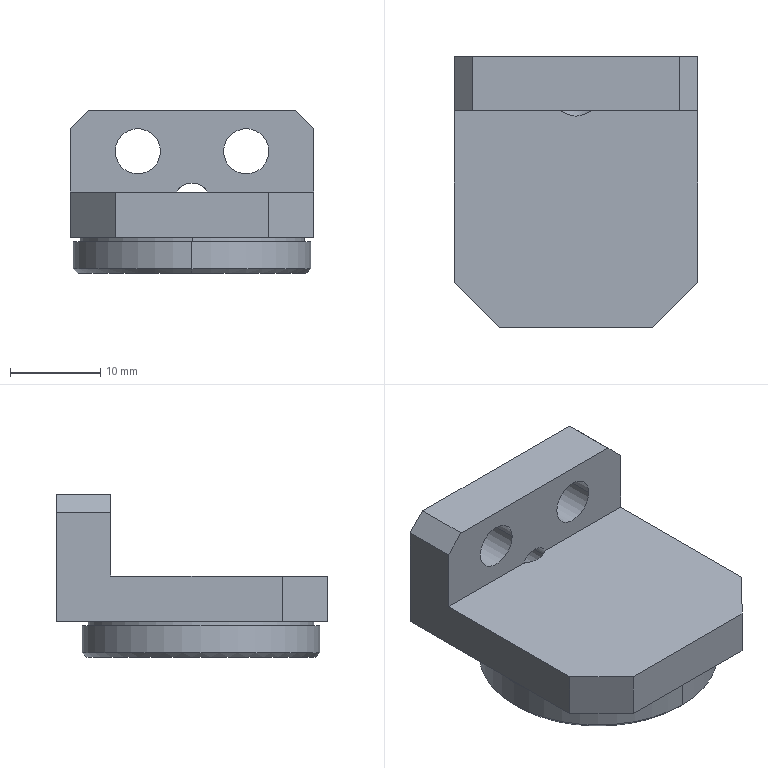Part | NX | 1 solid | 28 faces | box 27 x 30 x 18 mm | volume 7179 mm3 | plane 14 | cylinder 10 | cone 4 | commonest cylinder face diameters 5 x4 4 x2 25 x2 26.29 x2
STEP:
#1=CARTESIAN_POINT('',(0.,0.145,-17.5));
#2=VERTEX_POINT('',#1);
#3=CARTESIAN_POINT('',(0.,-26.145,-17.5));
#4=VERTEX_POINT('',#3);
#5=CARTESIAN_POINT('',(0.,-13.,-17.5));
#6=DIRECTION('',(0.,0.,1.));
#7=DIRECTION('',(0.,-1.,0.));
#8=AXIS2_PLACEMENT_3D('',#5,#6,#7);
#9=CIRCLE('',#8,13.145);
#10=EDGE_CURVE('',#2,#4,#9,.T.);
#11=ORIENTED_EDGE('',*,*,#10,.T.);
#12=CARTESIAN_POINT('',(0.,-26.145,-14.5));
#13=VERTEX_POINT('',#12);
#14=CARTESIAN_POINT('',(0.,-26.145,-18.));
#15=DIRECTION('',(0.,0.,1.));
#16=VECTOR('',#15,1000.);
#17=LINE('',#14,#16);
#18=EDGE_CURVE('',#13,#4,#17,.F.);
#19=ORIENTED_EDGE('',*,*,#18,.F.);
#20=CARTESIAN_POINT('',(0.,0.145,-14.5));
#21=VERTEX_POINT('',#20);
#22=CARTESIAN_POINT('',(0.,-13.,-14.5));
#23=DIRECTION('',(0.,0.,-1.));
#24=DIRECTION('',(0.,-1.,0.));
#25=AXIS2_PLACEMENT_3D('',#22,#23,#24);
#26=CIRCLE('',#25,13.145);
#27=EDGE_CURVE('',#13,#21,#26,.T.);
#28=ORIENTED_EDGE('',*,*,#27,.T.);
#29=CARTESIAN_POINT('',(0.,0.145,-18.));
#30=DIRECTION('',(0.,0.,1.));
#31=VECTOR('',#30,1000.);
#32=LINE('',#29,#31);
#33=EDGE_CURVE('',#21,#2,#32,.F.);
#34=ORIENTED_EDGE('',*,*,#33,.T.);
#35=EDGE_LOOP('',(#11,#19,#28,#34));
#36=FACE_BOUND('',#35,.T.);
#37=CARTESIAN_POINT('',(0.,-13.,-18.));
#38=DIRECTION('',(0.,0.,1.));
#39=DIRECTION('',(0.,-1.,0.));
#40=AXIS2_PLACEMENT_3D('',#37,#38,#39);
#41=CYLINDRICAL_SURFACE('',#40,13.145);
#42=ADVANCED_FACE('',(#36),#41,.T.);
#43=CARTESIAN_POINT('',(0.,-25.645,-18.));
#44=VERTEX_POINT('',#43);
#45=CARTESIAN_POINT('',(0.,-0.355,-18.));
#46=VERTEX_POINT('',#45);
#47=CARTESIAN_POINT('',(0.,-13.,-18.));
#48=DIRECTION('',(0.,0.,-1.));
#49=DIRECTION('',(0.,-1.,0.));
#50=AXIS2_PLACEMENT_3D('',#47,#48,#49);
#51=CIRCLE('',#50,12.645);
#52=EDGE_CURVE('',#44,#46,#51,.T.);
#53=ORIENTED_EDGE('',*,*,#52,.F.);
#54=CARTESIAN_POINT('',(0.,-25.645,-18.));
#55=DIRECTION('',(0.,-0.7071,0.7071));
#56=VECTOR('',#55,1000.);
#57=LINE('',#54,#56);
#58=EDGE_CURVE('',#4,#44,#57,.F.);
#59=ORIENTED_EDGE('',*,*,#58,.F.);
#60=ORIENTED_EDGE('',*,*,#10,.F.);
#61=CARTESIAN_POINT('',(0.,-0.355,-18.));
#62=DIRECTION('',(0.,0.7071,0.7071));
#63=VECTOR('',#62,1000.);
#64=LINE('',#61,#63);
#65=EDGE_CURVE('',#2,#46,#64,.F.);
#66=ORIENTED_EDGE('',*,*,#65,.T.);
#67=EDGE_LOOP('',(#53,#59,#60,#66));
#68=FACE_BOUND('',#67,.T.);
#69=CARTESIAN_POINT('',(0.,-13.,-18.));
#70=DIRECTION('',(0.,0.,1.));
#71=DIRECTION('',(0.,-1.,0.));
#72=AXIS2_PLACEMENT_3D('',#69,#70,#71);
#73=CONICAL_SURFACE('',#72,12.645,0.7854);
#74=ADVANCED_FACE('',(#68),#73,.T.);
#75=CARTESIAN_POINT('',(0.,-25.5,-14.5));
#76=VERTEX_POINT('',#75);
#77=CARTESIAN_POINT('',(0.,-0.5,-14.5));
#78=VERTEX_POINT('',#77);
#79=CARTESIAN_POINT('',(0.,-13.,-14.5));
#80=DIRECTION('',(0.,0.,-1.));
#81=DIRECTION('',(0.,-1.,0.));
#82=AXIS2_PLACEMENT_3D('',#79,#80,#81);
#83=CIRCLE('',#82,12.5);
#84=EDGE_CURVE('',#76,#78,#83,.T.);
#85=ORIENTED_EDGE('',*,*,#84,.F.);
#86=CARTESIAN_POINT('',(0.,-25.5,-14.));
#87=VERTEX_POINT('',#86);
#88=CARTESIAN_POINT('',(0.,-25.5,-14.5));
#89=DIRECTION('',(0.,0.,1.));
#90=VECTOR('',#89,1000.);
#91=LINE('',#88,#90);
#92=EDGE_CURVE('',#87,#76,#91,.F.);
#93=ORIENTED_EDGE('',*,*,#92,.F.);
#94=CARTESIAN_POINT('',(0.,-0.5,-14.));
#95=VERTEX_POINT('',#94);
#96=CARTESIAN_POINT('',(0.,-13.,-14.));
#97=DIRECTION('',(0.,0.,-1.));
#98=DIRECTION('',(0.,-1.,0.));
#99=AXIS2_PLACEMENT_3D('',#96,#97,#98);
#100=CIRCLE('',#99,12.5);
#101=EDGE_CURVE('',#87,#95,#100,.T.);
#102=ORIENTED_EDGE('',*,*,#101,.T.);
#103=CARTESIAN_POINT('',(0.,-0.5,-14.5));
#104=DIRECTION('',(0.,0.,1.));
#105=VECTOR('',#104,1000.);
#106=LINE('',#103,#105);
#107=EDGE_CURVE('',#95,#78,#106,.F.);
#108=ORIENTED_EDGE('',*,*,#107,.T.);
#109=EDGE_LOOP('',(#85,#93,#102,#108));
#110=FACE_BOUND('',#109,.T.);
#111=CARTESIAN_POINT('',(0.,-13.,-14.5));
#112=DIRECTION('',(0.,0.,1.));
#113=DIRECTION('',(0.,-1.,0.));
#114=AXIS2_PLACEMENT_3D('',#111,#112,#113);
#115=CYLINDRICAL_SURFACE('',#114,12.5);
#116=ADVANCED_FACE('',(#110),#115,.T.);
#117=CARTESIAN_POINT('',(-2.,-3.,-10.));
#118=VERTEX_POINT('',#117);
#119=CARTESIAN_POINT('',(-1.732,-3.,-9.));
#120=VERTEX_POINT('',#119);
#121=CARTESIAN_POINT('',(0.,-3.,-10.));
#122=DIRECTION('',(0.,1.,0.));
#123=DIRECTION('',(1.,0.,0.));
#124=AXIS2_PLACEMENT_3D('',#121,#122,#123);
#125=CIRCLE('',#124,2.);
#126=EDGE_CURVE('',#118,#120,#125,.T.);
#127=ORIENTED_EDGE('',*,*,#126,.F.);
#128=CARTESIAN_POINT('',(-2.,3.,-10.));
#129=VERTEX_POINT('',#128);
#130=CARTESIAN_POINT('',(-2.,3.,-10.));
#131=DIRECTION('',(0.,1.,0.));
#132=VECTOR('',#131,1000.);
#133=LINE('',#130,#132);
#134=EDGE_CURVE('',#129,#118,#133,.F.);
#135=ORIENTED_EDGE('',*,*,#134,.F.);
#136=CARTESIAN_POINT('',(2.,3.,-10.));
#137=VERTEX_POINT('',#136);
#138=CARTESIAN_POINT('',(0.,3.,-10.));
#139=DIRECTION('',(0.,1.,0.));
#140=DIRECTION('',(1.,0.,0.));
#141=AXIS2_PLACEMENT_3D('',#138,#139,#140);
#142=CIRCLE('',#141,2.);
#143=EDGE_CURVE('',#129,#137,#142,.T.);
#144=ORIENTED_EDGE('',*,*,#143,.T.);
#145=CARTESIAN_POINT('',(2.,-3.,-10.));
#146=VERTEX_POINT('',#145);
#147=CARTESIAN_POINT('',(2.,3.,-10.));
#148=DIRECTION('',(0.,1.,0.));
#149=VECTOR('',#148,1000.);
#150=LINE('',#147,#149);
#151=EDGE_CURVE('',#137,#146,#150,.F.);
#152=ORIENTED_EDGE('',*,*,#151,.T.);
#153=CARTESIAN_POINT('',(1.732,-3.,-9.));
#154=VERTEX_POINT('',#153);
#155=CARTESIAN_POINT('',(0.,-3.,-10.));
#156=DIRECTION('',(0.,1.,0.));
#157=DIRECTION('',(1.,0.,0.));
#158=AXIS2_PLACEMENT_3D('',#155,#156,#157);
#159=CIRCLE('',#158,2.);
#160=EDGE_CURVE('',#154,#146,#159,.T.);
#161=ORIENTED_EDGE('',*,*,#160,.F.);
#162=CARTESIAN_POINT('',(0.,-3.,-10.));
#163=DIRECTION('',(0.,1.,0.));
#164=DIRECTION('',(1.,0.,0.));
#165=AXIS2_PLACEMENT_3D('',#162,#163,#164);
#166=CIRCLE('',#165,2.);
#167=EDGE_CURVE('',#120,#154,#166,.T.);
#168=ORIENTED_EDGE('',*,*,#167,.F.);
#169=EDGE_LOOP('',(#127,#135,#144,#152,#161,#168));
#170=FACE_BOUND('',#169,.T.);
#171=CARTESIAN_POINT('',(0.,3.,-10.));
#172=DIRECTION('',(0.,1.,0.));
#173=DIRECTION('',(-1.,0.,0.));
#174=AXIS2_PLACEMENT_3D('',#171,#172,#173);
#175=CYLINDRICAL_SURFACE('',#174,2.);
#176=ADVANCED_FACE('',(#170),#175,.F.);
#177=CARTESIAN_POINT('',(0.,-4.202,-10.));
#178=VERTEX_POINT('',#177);
#179=CARTESIAN_POINT('',(2.,-3.,-10.));
#180=DIRECTION('',(0.8572,0.515,0.));
#181=VECTOR('',#180,1000.);
#182=LINE('',#179,#181);
#183=EDGE_CURVE('',#146,#178,#182,.F.);
#184=ORIENTED_EDGE('',*,*,#183,.T.);
#185=CARTESIAN_POINT('',(-2.,-3.,-10.));
#186=DIRECTION('',(-0.8572,0.515,0.));
#187=VECTOR('',#186,1000.);
#188=LINE('',#185,#187);
#189=EDGE_CURVE('',#118,#178,#188,.F.);
#190=ORIENTED_EDGE('',*,*,#189,.F.);
#191=ORIENTED_EDGE('',*,*,#126,.T.);
#192=CARTESIAN_POINT('',(1.732,-3.,-9.));
#193=CARTESIAN_POINT('',(1.184,-3.285,-9.));
#194=CARTESIAN_POINT('',(-0.003576,-3.917,-9.));
#195=CARTESIAN_POINT('',(-1.185,-3.285,-9.));
#196=CARTESIAN_POINT('',(-1.732,-3.,-9.));
#197=B_SPLINE_CURVE_WITH_KNOTS('',3,(#192,#193,#194,#195,#196),.UNSPECIFIED.,.F.,.F.,(4,1,4),(0.,0.001852,0.003703),.UNSPECIFIED.);
#198=EDGE_CURVE('',#154,#120,#197,.T.);
#199=ORIENTED_EDGE('',*,*,#198,.F.);
#200=ORIENTED_EDGE('',*,*,#160,.T.);
#201=EDGE_LOOP('',(#184,#190,#191,#199,#200));
#202=FACE_BOUND('',#201,.T.);
#203=CARTESIAN_POINT('',(0.,-3.,-10.));
#204=DIRECTION('',(0.,1.,0.));
#205=DIRECTION('',(-1.,0.,0.));
#206=AXIS2_PLACEMENT_3D('',#203,#204,#205);
#207=CONICAL_SURFACE('',#206,2.,1.03);
#208=ADVANCED_FACE('',(#202),#207,.F.);
#209=CARTESIAN_POINT('',(-8.5,-3.,-4.5));
#210=VERTEX_POINT('',#209);
#211=CARTESIAN_POINT('',(-3.5,-3.,-4.5));
#212=VERTEX_POINT('',#211);
#213=CARTESIAN_POINT('',(-6.,-3.,-4.5));
#214=DIRECTION('',(0.,1.,0.));
#215=DIRECTION('',(1.,0.,0.));
#216=AXIS2_PLACEMENT_3D('',#213,#214,#215);
#217=CIRCLE('',#216,2.5);
#218=EDGE_CURVE('',#210,#212,#217,.T.);
#219=ORIENTED_EDGE('',*,*,#218,.F.);
#220=CARTESIAN_POINT('',(-8.5,3.,-4.5));
#221=VERTEX_POINT('',#220);
#222=CARTESIAN_POINT('',(-8.5,-6.,-4.5));
#223=DIRECTION('',(0.,1.,0.));
#224=VECTOR('',#223,1000.);
#225=LINE('',#222,#224);
#226=EDGE_CURVE('',#221,#210,#225,.F.);
#227=ORIENTED_EDGE('',*,*,#226,.F.);
#228=CARTESIAN_POINT('',(-3.5,3.,-4.5));
#229=VERTEX_POINT('',#228);
#230=CARTESIAN_POINT('',(-6.,3.,-4.5));
#231=DIRECTION('',(0.,1.,0.));
#232=DIRECTION('',(1.,0.,0.));
#233=AXIS2_PLACEMENT_3D('',#230,#231,#232);
#234=CIRCLE('',#233,2.5);
#235=EDGE_CURVE('',#221,#229,#234,.T.);
#236=ORIENTED_EDGE('',*,*,#235,.T.);
#237=CARTESIAN_POINT('',(-3.5,-6.,-4.5));
#238=DIRECTION('',(0.,1.,0.));
#239=VECTOR('',#238,1000.);
#240=LINE('',#237,#239);
#241=EDGE_CURVE('',#229,#212,#240,.F.);
#242=ORIENTED_EDGE('',*,*,#241,.T.);
#243=EDGE_LOOP('',(#219,#227,#236,#242));
#244=FACE_BOUND('',#243,.T.);
#245=CARTESIAN_POINT('',(-6.,-6.,-4.5));
#246=DIRECTION('',(0.,1.,0.));
#247=DIRECTION('',(-1.,0.,0.));
#248=AXIS2_PLACEMENT_3D('',#245,#246,#247);
#249=CYLINDRICAL_SURFACE('',#248,2.5);
#250=ADVANCED_FACE('',(#244),#249,.F.);
#251=CARTESIAN_POINT('',(3.5,-3.,-4.5));
#252=VERTEX_POINT('',#251);
#253=CARTESIAN_POINT('',(8.5,-3.,-4.5));
#254=VERTEX_POINT('',#253);
#255=CARTESIAN_POINT('',(6.,-3.,-4.5));
#256=DIRECTION('',(0.,1.,0.));
#257=DIRECTION('',(1.,0.,0.));
#258=AXIS2_PLACEMENT_3D('',#255,#256,#257);
#259=CIRCLE('',#258,2.5);
#260=EDGE_CURVE('',#252,#254,#259,.T.);
#261=ORIENTED_EDGE('',*,*,#260,.F.);
#262=CARTESIAN_POINT('',(3.5,3.,-4.5));
#263=VERTEX_POINT('',#262);
#264=CARTESIAN_POINT('',(3.5,-6.,-4.5));
#265=DIRECTION('',(0.,1.,0.));
#266=VECTOR('',#265,1000.);
#267=LINE('',#264,#266);
#268=EDGE_CURVE('',#263,#252,#267,.F.);
#269=ORIENTED_EDGE('',*,*,#268,.F.);
#270=CARTESIAN_POINT('',(8.5,3.,-4.5));
#271=VERTEX_POINT('',#270);
#272=CARTESIAN_POINT('',(6.,3.,-4.5));
#273=DIRECTION('',(0.,1.,0.));
#274=DIRECTION('',(1.,0.,0.));
#275=AXIS2_PLACEMENT_3D('',#272,#273,#274);
#276=CIRCLE('',#275,2.5);
#277=EDGE_CURVE('',#263,#271,#276,.T.);
#278=ORIENTED_EDGE('',*,*,#277,.T.);
#279=CARTESIAN_POINT('',(8.5,-6.,-4.5));
#280=DIRECTION('',(0.,1.,0.));
#281=VECTOR('',#280,1000.);
#282=LINE('',#279,#281);
#283=EDGE_CURVE('',#271,#254,#282,.F.);
#284=ORIENTED_EDGE('',*,*,#283,.T.);
#285=EDGE_LOOP('',(#261,#269,#278,#284));
#286=FACE_BOUND('',#285,.T.);
#287=CARTESIAN_POINT('',(6.,-6.,-4.5));
#288=DIRECTION('',(0.,1.,0.));
#289=DIRECTION('',(-1.,0.,0.));
#290=AXIS2_PLACEMENT_3D('',#287,#288,#289);
#291=CYLINDRICAL_SURFACE('',#290,2.5);
#292=ADVANCED_FACE('',(#286),#291,.F.);
#293=CARTESIAN_POINT('',(-13.5,-22.,-9.));
#294=VERTEX_POINT('',#293);
#295=CARTESIAN_POINT('',(-13.5,-3.,-9.));
#296=VERTEX_POINT('',#295);
#297=CARTESIAN_POINT('',(-13.5,-27.,-9.));
#298=DIRECTION('',(0.,1.,0.));
#299=VECTOR('',#298,1000.);
#300=LINE('',#297,#299);
#301=EDGE_CURVE('',#294,#296,#300,.T.);
#302=ORIENTED_EDGE('',*,*,#301,.F.);
#303=CARTESIAN_POINT('',(-8.5,-27.,-9.));
#304=VERTEX_POINT('',#303);
#305=CARTESIAN_POINT('',(-13.5,-22.,-9.));
#306=DIRECTION('',(0.7071,-0.7071,0.));
#307=VECTOR('',#306,1000.);
#308=LINE('',#305,#307);
#309=EDGE_CURVE('',#294,#304,#308,.T.);
#310=ORIENTED_EDGE('',*,*,#309,.T.);
#311=CARTESIAN_POINT('',(8.5,-27.,-9.));
#312=VERTEX_POINT('',#311);
#313=CARTESIAN_POINT('',(-13.5,-27.,-9.));
#314=DIRECTION('',(-1.,0.,0.));
#315=VECTOR('',#314,1000.);
#316=LINE('',#313,#315);
#317=EDGE_CURVE('',#312,#304,#316,.T.);
#318=ORIENTED_EDGE('',*,*,#317,.F.);
#319=CARTESIAN_POINT('',(13.5,-22.,-9.));
#320=VERTEX_POINT('',#319);
#321=CARTESIAN_POINT('',(8.5,-27.,-9.));
#322=DIRECTION('',(0.7071,0.7071,0.));
#323=VECTOR('',#322,1000.);
#324=LINE('',#321,#323);
#325=EDGE_CURVE('',#312,#320,#324,.T.);
#326=ORIENTED_EDGE('',*,*,#325,.T.);
#327=CARTESIAN_POINT('',(13.5,-3.,-9.));
#328=VERTEX_POINT('',#327);
#329=CARTESIAN_POINT('',(13.5,-27.,-9.));
#330=DIRECTION('',(0.,-1.,0.));
#331=VECTOR('',#330,1000.);
#332=LINE('',#329,#331);
#333=EDGE_CURVE('',#328,#320,#332,.T.);
#334=ORIENTED_EDGE('',*,*,#333,.F.);
#335=CARTESIAN_POINT('',(13.5,-3.,-9.));
#336=DIRECTION('',(1.,0.,0.));
#337=VECTOR('',#336,1000.);
#338=LINE('',#335,#337);
#339=EDGE_CURVE('',#154,#328,#338,.T.);
#340=ORIENTED_EDGE('',*,*,#339,.F.);
#341=ORIENTED_EDGE('',*,*,#198,.T.);
#342=CARTESIAN_POINT('',(13.5,-3.,-9.));
#343=DIRECTION('',(1.,0.,0.));
#344=VECTOR('',#343,1000.);
#345=LINE('',#342,#344);
#346=EDGE_CURVE('',#296,#120,#345,.T.);
#347=ORIENTED_EDGE('',*,*,#346,.F.);
#348=EDGE_LOOP('',(#302,#310,#318,#326,#334,#340,#341,#347));
#349=FACE_BOUND('',#348,.T.);
#350=CARTESIAN_POINT('',(0.,-13.,-9.));
#351=DIRECTION('',(0.,0.,-1.));
#352=DIRECTION('',(0.,1.,0.));
#353=AXIS2_PLACEMENT_3D('',#350,#351,#352);
#354=PLANE('',#353);
#355=ADVANCED_FACE('',(#349),#354,.F.);
#356=ORIENTED_EDGE('',*,*,#333,.T.);
#357=CARTESIAN_POINT('',(13.5,-22.,-14.));
#358=VERTEX_POINT('',#357);
#359=CARTESIAN_POINT('',(13.5,-22.,-14.));
#360=DIRECTION('',(0.,0.,-1.));
#361=VECTOR('',#360,1000.);
#362=LINE('',#359,#361);
#363=EDGE_CURVE('',#320,#358,#362,.T.);
#364=ORIENTED_EDGE('',*,*,#363,.T.);
#365=CARTESIAN_POINT('',(13.5,3.,-14.));
#366=VERTEX_POINT('',#365);
#367=CARTESIAN_POINT('',(13.5,-27.,-14.));
#368=DIRECTION('',(0.,-1.,0.));
#369=VECTOR('',#368,1000.);
#370=LINE('',#367,#369);
#371=EDGE_CURVE('',#366,#358,#370,.T.);
#372=ORIENTED_EDGE('',*,*,#371,.F.);
#373=CARTESIAN_POINT('',(13.5,3.,-2.));
#374=VERTEX_POINT('',#373);
#375=CARTESIAN_POINT('',(13.5,3.,-14.));
#376=DIRECTION('',(0.,0.,1.));
#377=VECTOR('',#376,1000.);
#378=LINE('',#375,#377);
#379=EDGE_CURVE('',#366,#374,#378,.T.);
#380=ORIENTED_EDGE('',*,*,#379,.T.);
#381=CARTESIAN_POINT('',(13.5,-3.,-2.));
#382=VERTEX_POINT('',#381);
#383=CARTESIAN_POINT('',(13.5,-27.,-2.));
#384=DIRECTION('',(0.,-1.,0.));
#385=VECTOR('',#384,1000.);
#386=LINE('',#383,#385);
#387=EDGE_CURVE('',#374,#382,#386,.T.);
#388=ORIENTED_EDGE('',*,*,#387,.T.);
#389=CARTESIAN_POINT('',(13.5,-3.,0.));
#390=DIRECTION('',(0.,0.,-1.));
#391=VECTOR('',#390,1000.);
#392=LINE('',#389,#391);
#393=EDGE_CURVE('',#382,#328,#392,.T.);
#394=ORIENTED_EDGE('',*,*,#393,.T.);
#395=EDGE_LOOP('',(#356,#364,#372,#380,#388,#394));
#396=FACE_BOUND('',#395,.T.);
#397=CARTESIAN_POINT('',(13.5,-27.,-14.));
#398=DIRECTION('',(-1.,0.,0.));
#399=DIRECTION('',(0.,-1.,0.));
#400=AXIS2_PLACEMENT_3D('',#397,#398,#399);
#401=PLANE('',#400);
#402=ADVANCED_FACE('',(#396),#401,.F.);
#403=ORIENTED_EDGE('',*,*,#317,.T.);
#404=CARTESIAN_POINT('',(-8.5,-27.,-14.));
#405=VERTEX_POINT('',#404);
#406=CARTESIAN_POINT('',(-8.5,-27.,-14.));
#407=DIRECTION('',(0.,0.,-1.));
#408=VECTOR('',#407,1000.);
#409=LINE('',#406,#408);
#410=EDGE_CURVE('',#304,#405,#409,.T.);
#411=ORIENTED_EDGE('',*,*,#410,.T.);
#412=CARTESIAN_POINT('',(8.5,-27.,-14.));
#413=VERTEX_POINT('',#412);
#414=CARTESIAN_POINT('',(-13.5,-27.,-14.));
#415=DIRECTION('',(-1.,0.,0.));
#416=VECTOR('',#415,1000.);
#417=LINE('',#414,#416);
#418=EDGE_CURVE('',#413,#405,#417,.T.);
#419=ORIENTED_EDGE('',*,*,#418,.F.);
#420=CARTESIAN_POINT('',(8.5,-27.,-14.));
#421=DIRECTION('',(0.,0.,1.));
#422=VECTOR('',#421,1000.);
#423=LINE('',#420,#422);
#424=EDGE_CURVE('',#413,#312,#423,.T.);
#425=ORIENTED_EDGE('',*,*,#424,.T.);
#426=EDGE_LOOP('',(#403,#411,#419,#425));
#427=FACE_BOUND('',#426,.T.);
#428=CARTESIAN_POINT('',(-13.5,-27.,-14.));
#429=DIRECTION('',(0.,1.,0.));
#430=DIRECTION('',(-1.,0.,0.));
#431=AXIS2_PLACEMENT_3D('',#428,#429,#430);
#432=PLANE('',#431);
#433=ADVANCED_FACE('',(#427),#432,.F.);
#434=CARTESIAN_POINT('',(-13.5,-22.,-14.));
#435=VERTEX_POINT('',#434);
#436=CARTESIAN_POINT('',(-13.5,3.,-14.));
#437=VERTEX_POINT('',#436);
#438=CARTESIAN_POINT('',(-13.5,-27.,-14.));
#439=DIRECTION('',(0.,1.,0.));
#440=VECTOR('',#439,1000.);
#441=LINE('',#438,#440);
#442=EDGE_CURVE('',#435,#437,#441,.T.);
#443=ORIENTED_EDGE('',*,*,#442,.F.);
#444=CARTESIAN_POINT('',(-13.5,-22.,-14.));
#445=DIRECTION('',(0.,0.,1.));
#446=VECTOR('',#445,1000.);
#447=LINE('',#444,#446);
#448=EDGE_CURVE('',#435,#294,#447,.T.);
#449=ORIENTED_EDGE('',*,*,#448,.T.);
#450=ORIENTED_EDGE('',*,*,#301,.T.);
#451=CARTESIAN_POINT('',(-13.5,-3.,-2.));
#452=VERTEX_POINT('',#451);
#453=CARTESIAN_POINT('',(-13.5,-3.,0.));
#454=DIRECTION('',(0.,0.,-1.));
#455=VECTOR('',#454,1000.);
#456=LINE('',#453,#455);
#457=EDGE_CURVE('',#452,#296,#456,.T.);
#458=ORIENTED_EDGE('',*,*,#457,.F.);
#459=CARTESIAN_POINT('',(-13.5,3.,-2.));
#460=VERTEX_POINT('',#459);
#461=CARTESIAN_POINT('',(-13.5,-27.,-2.));
#462=DIRECTION('',(0.,1.,0.));
#463=VECTOR('',#462,1000.);
#464=LINE('',#461,#463);
#465=EDGE_CURVE('',#452,#460,#464,.T.);
#466=ORIENTED_EDGE('',*,*,#465,.T.);
#467=CARTESIAN_POINT('',(-13.5,3.,-14.));
#468=DIRECTION('',(0.,0.,1.));
#469=VECTOR('',#468,1000.);
#470=LINE('',#467,#469);
#471=EDGE_CURVE('',#437,#460,#470,.T.);
#472=ORIENTED_EDGE('',*,*,#471,.F.);
#473=EDGE_LOOP('',(#443,#449,#450,#458,#466,#472));
#474=FACE_BOUND('',#473,.T.);
#475=CARTESIAN_POINT('',(-13.5,-27.,-14.));
#476=DIRECTION('',(1.,0.,0.));
#477=DIRECTION('',(0.,1.,0.));
#478=AXIS2_PLACEMENT_3D('',#475,#476,#477);
#479=PLANE('',#478);
#480=ADVANCED_FACE('',(#474),#479,.F.);
#481=CARTESIAN_POINT('',(0.,3.,-10.));
#482=DIRECTION('',(0.,1.,0.));
#483=DIRECTION('',(1.,0.,0.));
#484=AXIS2_PLACEMENT_3D('',#481,#482,#483);
#485=CIRCLE('',#484,2.);
#486=EDGE_CURVE('',#137,#129,#485,.T.);
#487=ORIENTED_EDGE('',*,*,#486,.F.);
#488=ORIENTED_EDGE('',*,*,#143,.F.);
#489=EDGE_LOOP('',(#487,#488));
#490=FACE_BOUND('',#489,.T.);
#491=CARTESIAN_POINT('',(-6.,3.,-4.5));
#492=DIRECTION('',(0.,1.,0.));
#493=DIRECTION('',(1.,0.,0.));
#494=AXIS2_PLACEMENT_3D('',#491,#492,#493);
#495=CIRCLE('',#494,2.5);
#496=EDGE_CURVE('',#229,#221,#495,.T.);
#497=ORIENTED_EDGE('',*,*,#496,.F.);
#498=ORIENTED_EDGE('',*,*,#235,.F.);
#499=EDGE_LOOP('',(#497,#498));
#500=FACE_BOUND('',#499,.T.);
#501=CARTESIAN_POINT('',(6.,3.,-4.5));
#502=DIRECTION('',(0.,1.,0.));
#503=DIRECTION('',(1.,0.,0.));
#504=AXIS2_PLACEMENT_3D('',#501,#502,#503);
#505=CIRCLE('',#504,2.5);
#506=EDGE_CURVE('',#271,#263,#505,.T.);
#507=ORIENTED_EDGE('',*,*,#506,.F.);
#508=ORIENTED_EDGE('',*,*,#277,.F.);
#509=EDGE_LOOP('',(#507,#508));
#510=FACE_BOUND('',#509,.T.);
#511=ORIENTED_EDGE('',*,*,#471,.T.);
#512=CARTESIAN_POINT('',(-11.5,3.,0.));
#513=VERTEX_POINT('',#512);
#514=CARTESIAN_POINT('',(-11.5,3.,0.));
#515=DIRECTION('',(0.7071,0.,0.7071));
#516=VECTOR('',#515,1000.);
#517=LINE('',#514,#516);
#518=EDGE_CURVE('',#460,#513,#517,.T.);
#519=ORIENTED_EDGE('',*,*,#518,.T.);
#520=CARTESIAN_POINT('',(11.5,3.,0.));
#521=VERTEX_POINT('',#520);
#522=CARTESIAN_POINT('',(13.5,3.,0.));
#523=DIRECTION('',(-1.,0.,0.));
#524=VECTOR('',#523,1000.);
#525=LINE('',#522,#524);
#526=EDGE_CURVE('',#521,#513,#525,.T.);
#527=ORIENTED_EDGE('',*,*,#526,.F.);
#528=CARTESIAN_POINT('',(11.5,3.,0.));
#529=DIRECTION('',(0.7071,0.,-0.7071));
#530=VECTOR('',#529,1000.);
#531=LINE('',#528,#530);
#532=EDGE_CURVE('',#521,#374,#531,.T.);
#533=ORIENTED_EDGE('',*,*,#532,.T.);
#534=ORIENTED_EDGE('',*,*,#379,.F.);
#535=CARTESIAN_POINT('',(-13.5,3.,-14.));
#536=DIRECTION('',(1.,0.,0.));
#537=VECTOR('',#536,1000.);
#538=LINE('',#535,#537);
#539=EDGE_CURVE('',#437,#366,#538,.T.);
#540=ORIENTED_EDGE('',*,*,#539,.F.);
#541=EDGE_LOOP('',(#511,#519,#527,#533,#534,#540));
#542=FACE_BOUND('',#541,.T.);
#543=CARTESIAN_POINT('',(-13.5,3.,-14.));
#544=DIRECTION('',(0.,-1.,0.));
#545=DIRECTION('',(1.,0.,0.));
#546=AXIS2_PLACEMENT_3D('',#543,#544,#545);
#547=PLANE('',#546);
#548=ADVANCED_FACE('',(#490,#500,#510,#542),#547,.F.);
#549=ORIENTED_EDGE('',*,*,#418,.T.);
#550=CARTESIAN_POINT('',(-11.25,-24.25,-14.));
#551=DIRECTION('',(-0.7071,0.7071,0.));
#552=VECTOR('',#551,1000.);
#553=LINE('',#550,#552);
#554=EDGE_CURVE('',#405,#435,#553,.T.);
#555=ORIENTED_EDGE('',*,*,#554,.T.);
#556=ORIENTED_EDGE('',*,*,#442,.T.);
#557=ORIENTED_EDGE('',*,*,#539,.T.);
#558=ORIENTED_EDGE('',*,*,#371,.T.);
#559=CARTESIAN_POINT('',(11.25,-24.25,-14.));
#560=DIRECTION('',(-0.7071,-0.7071,0.));
#561=VECTOR('',#560,1000.);
#562=LINE('',#559,#561);
#563=EDGE_CURVE('',#358,#413,#562,.T.);
#564=ORIENTED_EDGE('',*,*,#563,.T.);
#565=EDGE_LOOP('',(#549,#555,#556,#557,#558,#564));
#566=FACE_BOUND('',#565,.T.);
#567=CARTESIAN_POINT('',(0.,-13.,-14.));
#568=DIRECTION('',(0.,0.,-1.));
#569=DIRECTION('',(0.,-1.,0.));
#570=AXIS2_PLACEMENT_3D('',#567,#568,#569);
#571=CIRCLE('',#570,12.5);
#572=EDGE_CURVE('',#95,#87,#571,.T.);
#573=ORIENTED_EDGE('',*,*,#572,.F.);
#574=ORIENTED_EDGE('',*,*,#101,.F.);
#575=EDGE_LOOP('',(#573,#574));
#576=FACE_BOUND('',#575,.T.);
#577=CARTESIAN_POINT('',(0.,-13.,-14.));
#578=DIRECTION('',(0.,0.,-1.));
#579=DIRECTION('',(0.,1.,0.));
#580=AXIS2_PLACEMENT_3D('',#577,#578,#579);
#581=PLANE('',#580);
#582=ADVANCED_FACE('',(#566,#576),#581,.T.);
#583=CARTESIAN_POINT('',(-6.,-3.,-4.5));
#584=DIRECTION('',(0.,1.,0.));
#585=DIRECTION('',(1.,0.,0.));
#586=AXIS2_PLACEMENT_3D('',#583,#584,#585);
#587=CIRCLE('',#586,2.5);
#588=EDGE_CURVE('',#212,#210,#587,.T.);
#589=ORIENTED_EDGE('',*,*,#588,.T.);
#590=ORIENTED_EDGE('',*,*,#218,.T.);
#591=EDGE_LOOP('',(#589,#590));
#592=FACE_BOUND('',#591,.T.);
#593=CARTESIAN_POINT('',(6.,-3.,-4.5));
#594=DIRECTION('',(0.,1.,0.));
#595=DIRECTION('',(1.,0.,0.));
#596=AXIS2_PLACEMENT_3D('',#593,#594,#595);
#597=CIRCLE('',#596,2.5);
#598=EDGE_CURVE('',#254,#252,#597,.T.);
#599=ORIENTED_EDGE('',*,*,#598,.T.);
#600=ORIENTED_EDGE('',*,*,#260,.T.);
#601=EDGE_LOOP('',(#599,#600));
#602=FACE_BOUND('',#601,.T.);
#603=CARTESIAN_POINT('',(-11.5,-3.,0.));
#604=VERTEX_POINT('',#603);
#605=CARTESIAN_POINT('',(11.5,-3.,0.));
#606=VERTEX_POINT('',#605);
#607=CARTESIAN_POINT('',(13.5,-3.,0.));
#608=DIRECTION('',(1.,0.,0.));
#609=VECTOR('',#608,1000.);
#610=LINE('',#607,#609);
#611=EDGE_CURVE('',#604,#606,#610,.T.);
#612=ORIENTED_EDGE('',*,*,#611,.F.);
#613=CARTESIAN_POINT('',(-11.5,-3.,0.));
#614=DIRECTION('',(-0.7071,0.,-0.7071));
#615=VECTOR('',#614,1000.);
#616=LINE('',#613,#615);
#617=EDGE_CURVE('',#604,#452,#616,.T.);
#618=ORIENTED_EDGE('',*,*,#617,.T.);
#619=ORIENTED_EDGE('',*,*,#457,.T.);
#620=ORIENTED_EDGE('',*,*,#346,.T.);
#621=ORIENTED_EDGE('',*,*,#167,.T.);
#622=ORIENTED_EDGE('',*,*,#339,.T.);
#623=ORIENTED_EDGE('',*,*,#393,.F.);
#624=CARTESIAN_POINT('',(11.5,-3.,0.));
#625=DIRECTION('',(-0.7071,0.,0.7071));
#626=VECTOR('',#625,1000.);
#627=LINE('',#624,#626);
#628=EDGE_CURVE('',#382,#606,#627,.T.);
#629=ORIENTED_EDGE('',*,*,#628,.T.);
#630=EDGE_LOOP('',(#612,#618,#619,#620,#621,#622,#623,#629));
#631=FACE_BOUND('',#630,.T.);
#632=CARTESIAN_POINT('',(13.5,-3.,0.));
#633=DIRECTION('',(0.,1.,0.));
#634=DIRECTION('',(-1.,0.,0.));
#635=AXIS2_PLACEMENT_3D('',#632,#633,#634);
#636=PLANE('',#635);
#637=ADVANCED_FACE('',(#592,#602,#631),#636,.F.);
#638=ORIENTED_EDGE('',*,*,#526,.T.);
#639=CARTESIAN_POINT('',(-11.5,-13.,0.));
#640=DIRECTION('',(0.,-1.,0.));
#641=VECTOR('',#640,1000.);
#642=LINE('',#639,#641);
#643=EDGE_CURVE('',#513,#604,#642,.T.);
#644=ORIENTED_EDGE('',*,*,#643,.T.);
#645=ORIENTED_EDGE('',*,*,#611,.T.);
#646=CARTESIAN_POINT('',(11.5,-13.,0.));
#647=DIRECTION('',(0.,1.,0.));
#648=VECTOR('',#647,1000.);
#649=LINE('',#646,#648);
#650=EDGE_CURVE('',#606,#521,#649,.T.);
#651=ORIENTED_EDGE('',*,*,#650,.T.);
#652=EDGE_LOOP('',(#638,#644,#645,#651));
#653=FACE_BOUND('',#652,.T.);
#654=CARTESIAN_POINT('',(0.,-13.,0.));
#655=DIRECTION('',(0.,0.,-1.));
#656=DIRECTION('',(0.,1.,0.));
#657=AXIS2_PLACEMENT_3D('',#654,#655,#656);
#658=PLANE('',#657);
#659=ADVANCED_FACE('',(#653),#658,.F.);
#660=ORIENTED_EDGE('',*,*,#268,.T.);
#661=ORIENTED_EDGE('',*,*,#598,.F.);
#662=ORIENTED_EDGE('',*,*,#283,.F.);
#663=ORIENTED_EDGE('',*,*,#506,.T.);
#664=EDGE_LOOP('',(#660,#661,#662,#663));
#665=FACE_BOUND('',#664,.T.);
#666=CARTESIAN_POINT('',(6.,-6.,-4.5));
#667=DIRECTION('',(0.,1.,0.));
#668=DIRECTION('',(-1.,0.,0.));
#669=AXIS2_PLACEMENT_3D('',#666,#667,#668);
#670=CYLINDRICAL_SURFACE('',#669,2.5);
#671=ADVANCED_FACE('',(#665),#670,.F.);
#672=ORIENTED_EDGE('',*,*,#226,.T.);
#673=ORIENTED_EDGE('',*,*,#588,.F.);
#674=ORIENTED_EDGE('',*,*,#241,.F.);
#675=ORIENTED_EDGE('',*,*,#496,.T.);
#676=EDGE_LOOP('',(#672,#673,#674,#675));
#677=FACE_BOUND('',#676,.T.);
#678=CARTESIAN_POINT('',(-6.,-6.,-4.5));
#679=DIRECTION('',(0.,1.,0.));
#680=DIRECTION('',(-1.,0.,0.));
#681=AXIS2_PLACEMENT_3D('',#678,#679,#680);
#682=CYLINDRICAL_SURFACE('',#681,2.5);
#683=ADVANCED_FACE('',(#677),#682,.F.);
#684=ORIENTED_EDGE('',*,*,#189,.T.);
#685=ORIENTED_EDGE('',*,*,#183,.F.);
#686=CARTESIAN_POINT('',(0.,-3.,-10.));
#687=DIRECTION('',(0.,1.,0.));
#688=DIRECTION('',(1.,0.,0.));
#689=AXIS2_PLACEMENT_3D('',#686,#687,#688);
#690=CIRCLE('',#689,2.);
#691=EDGE_CURVE('',#146,#118,#690,.T.);
#692=ORIENTED_EDGE('',*,*,#691,.T.);
#693=EDGE_LOOP('',(#684,#685,#692));
#694=FACE_BOUND('',#693,.T.);
#695=CARTESIAN_POINT('',(0.,-3.,-10.));
#696=DIRECTION('',(0.,1.,0.));
#697=DIRECTION('',(-1.,0.,0.));
#698=AXIS2_PLACEMENT_3D('',#695,#696,#697);
#699=CONICAL_SURFACE('',#698,2.,1.03);
#700=ADVANCED_FACE('',(#694),#699,.F.);
#701=ORIENTED_EDGE('',*,*,#134,.T.);
#702=ORIENTED_EDGE('',*,*,#691,.F.);
#703=ORIENTED_EDGE('',*,*,#151,.F.);
#704=ORIENTED_EDGE('',*,*,#486,.T.);
#705=EDGE_LOOP('',(#701,#702,#703,#704));
#706=FACE_BOUND('',#705,.T.);
#707=CARTESIAN_POINT('',(0.,3.,-10.));
#708=DIRECTION('',(0.,1.,0.));
#709=DIRECTION('',(-1.,0.,0.));
#710=AXIS2_PLACEMENT_3D('',#707,#708,#709);
#711=CYLINDRICAL_SURFACE('',#710,2.);
#712=ADVANCED_FACE('',(#706),#711,.F.);
#713=ORIENTED_EDGE('',*,*,#518,.F.);
#714=ORIENTED_EDGE('',*,*,#465,.F.);
#715=ORIENTED_EDGE('',*,*,#617,.F.);
#716=ORIENTED_EDGE('',*,*,#643,.F.);
#717=EDGE_LOOP('',(#713,#714,#715,#716));
#718=FACE_BOUND('',#717,.T.);
#719=CARTESIAN_POINT('',(-11.5,-13.,0.));
#720=DIRECTION('',(0.7071,0.,-0.7071));
#721=DIRECTION('',(0.,1.,0.));
#722=AXIS2_PLACEMENT_3D('',#719,#720,#721);
#723=PLANE('',#722);
#724=ADVANCED_FACE('',(#718),#723,.F.);
#725=ORIENTED_EDGE('',*,*,#628,.F.);
#726=ORIENTED_EDGE('',*,*,#387,.F.);
#727=ORIENTED_EDGE('',*,*,#532,.F.);
#728=ORIENTED_EDGE('',*,*,#650,.F.);
#729=EDGE_LOOP('',(#725,#726,#727,#728));
#730=FACE_BOUND('',#729,.T.);
#731=CARTESIAN_POINT('',(11.5,-13.,0.));
#732=DIRECTION('',(-0.7071,0.,-0.7071));
#733=DIRECTION('',(0.,-1.,0.));
#734=AXIS2_PLACEMENT_3D('',#731,#732,#733);
#735=PLANE('',#734);
#736=ADVANCED_FACE('',(#730),#735,.F.);
#737=ORIENTED_EDGE('',*,*,#554,.F.);
#738=ORIENTED_EDGE('',*,*,#410,.F.);
#739=ORIENTED_EDGE('',*,*,#309,.F.);
#740=ORIENTED_EDGE('',*,*,#448,.F.);
#741=EDGE_LOOP('',(#737,#738,#739,#740));
#742=FACE_BOUND('',#741,.T.);
#743=CARTESIAN_POINT('',(-13.5,-22.,-14.));
#744=DIRECTION('',(0.7071,0.7071,0.));
#745=DIRECTION('',(0.,0.,-1.));
#746=AXIS2_PLACEMENT_3D('',#743,#744,#745);
#747=PLANE('',#746);
#748=ADVANCED_FACE('',(#742),#747,.F.);
#749=ORIENTED_EDGE('',*,*,#563,.F.);
#750=ORIENTED_EDGE('',*,*,#363,.F.);
#751=ORIENTED_EDGE('',*,*,#325,.F.);
#752=ORIENTED_EDGE('',*,*,#424,.F.);
#753=EDGE_LOOP('',(#749,#750,#751,#752));
#754=FACE_BOUND('',#753,.T.);
#755=CARTESIAN_POINT('',(8.5,-27.,-14.));
#756=DIRECTION('',(-0.7071,0.7071,0.));
#757=DIRECTION('',(0.,0.,-1.));
#758=AXIS2_PLACEMENT_3D('',#755,#756,#757);
#759=PLANE('',#758);
#760=ADVANCED_FACE('',(#754),#759,.F.);
#761=CARTESIAN_POINT('',(0.,-13.,-14.5));
#762=DIRECTION('',(0.,0.,-1.));
#763=DIRECTION('',(0.,-1.,0.));
#764=AXIS2_PLACEMENT_3D('',#761,#762,#763);
#765=CIRCLE('',#764,12.5);
#766=EDGE_CURVE('',#78,#76,#765,.T.);
#767=ORIENTED_EDGE('',*,*,#766,.T.);
#768=ORIENTED_EDGE('',*,*,#84,.T.);
#769=EDGE_LOOP('',(#767,#768));
#770=FACE_BOUND('',#769,.T.);
#771=CARTESIAN_POINT('',(0.,-13.,-14.5));
#772=DIRECTION('',(0.,0.,-1.));
#773=DIRECTION('',(0.,-1.,0.));
#774=AXIS2_PLACEMENT_3D('',#771,#772,#773);
#775=CIRCLE('',#774,13.145);
#776=EDGE_CURVE('',#21,#13,#775,.T.);
#777=ORIENTED_EDGE('',*,*,#776,.F.);
#778=ORIENTED_EDGE('',*,*,#27,.F.);
#779=EDGE_LOOP('',(#777,#778));
#780=FACE_BOUND('',#779,.T.);
#781=CARTESIAN_POINT('',(0.,-12.,-14.5));
#782=DIRECTION('',(0.,0.,-1.));
#783=DIRECTION('',(0.,1.,0.));
#784=AXIS2_PLACEMENT_3D('',#781,#782,#783);
#785=PLANE('',#784);
#786=ADVANCED_FACE('',(#770,#780),#785,.F.);
#787=ORIENTED_EDGE('',*,*,#92,.T.);
#788=ORIENTED_EDGE('',*,*,#766,.F.);
#789=ORIENTED_EDGE('',*,*,#107,.F.);
#790=ORIENTED_EDGE('',*,*,#572,.T.);
#791=EDGE_LOOP('',(#787,#788,#789,#790));
#792=FACE_BOUND('',#791,.T.);
#793=CARTESIAN_POINT('',(0.,-13.,-14.5));
#794=DIRECTION('',(0.,0.,1.));
#795=DIRECTION('',(0.,-1.,0.));
#796=AXIS2_PLACEMENT_3D('',#793,#794,#795);
#797=CYLINDRICAL_SURFACE('',#796,12.5);
#798=ADVANCED_FACE('',(#792),#797,.T.);
#799=CARTESIAN_POINT('',(0.,-13.,-18.));
#800=DIRECTION('',(0.,0.,-1.));
#801=DIRECTION('',(0.,-1.,0.));
#802=AXIS2_PLACEMENT_3D('',#799,#800,#801);
#803=CIRCLE('',#802,12.645);
#804=EDGE_CURVE('',#46,#44,#803,.T.);
#805=ORIENTED_EDGE('',*,*,#804,.T.);
#806=ORIENTED_EDGE('',*,*,#52,.T.);
#807=EDGE_LOOP('',(#805,#806));
#808=FACE_BOUND('',#807,.T.);
#809=CARTESIAN_POINT('',(0.,-13.,-18.));
#810=DIRECTION('',(0.,0.,-1.));
#811=DIRECTION('',(0.,1.,0.));
#812=AXIS2_PLACEMENT_3D('',#809,#810,#811);
#813=PLANE('',#812);
#814=ADVANCED_FACE('',(#808),#813,.T.);
#815=ORIENTED_EDGE('',*,*,#58,.T.);
#816=ORIENTED_EDGE('',*,*,#804,.F.);
#817=ORIENTED_EDGE('',*,*,#65,.F.);
#818=CARTESIAN_POINT('',(0.,-13.,-17.5));
#819=DIRECTION('',(0.,0.,1.));
#820=DIRECTION('',(0.,-1.,0.));
#821=AXIS2_PLACEMENT_3D('',#818,#819,#820);
#822=CIRCLE('',#821,13.145);
#823=EDGE_CURVE('',#4,#2,#822,.T.);
#824=ORIENTED_EDGE('',*,*,#823,.F.);
#825=EDGE_LOOP('',(#815,#816,#817,#824));
#826=FACE_BOUND('',#825,.T.);
#827=CARTESIAN_POINT('',(0.,-13.,-18.));
#828=DIRECTION('',(0.,0.,1.));
#829=DIRECTION('',(0.,-1.,0.));
#830=AXIS2_PLACEMENT_3D('',#827,#828,#829);
#831=CONICAL_SURFACE('',#830,12.645,0.7854);
#832=ADVANCED_FACE('',(#826),#831,.T.);
#833=ORIENTED_EDGE('',*,*,#18,.T.);
#834=ORIENTED_EDGE('',*,*,#823,.T.);
#835=ORIENTED_EDGE('',*,*,#33,.F.);
#836=ORIENTED_EDGE('',*,*,#776,.T.);
#837=EDGE_LOOP('',(#833,#834,#835,#836));
#838=FACE_BOUND('',#837,.T.);
#839=CARTESIAN_POINT('',(0.,-13.,-18.));
#840=DIRECTION('',(0.,0.,1.));
#841=DIRECTION('',(0.,-1.,0.));
#842=AXIS2_PLACEMENT_3D('',#839,#840,#841);
#843=CYLINDRICAL_SURFACE('',#842,13.145);
#844=ADVANCED_FACE('',(#838),#843,.T.);
#845=CLOSED_SHELL('',(#42,#74,#116,#176,#208,#250,#292,#355,#402,#433,#480,#548,#582,#637,#659,#671,#683,#700,#712,#724,#736,#748,#760,#786,#798,#814,#832,#844));
#846=MANIFOLD_SOLID_BREP('',#845);
#847=(LENGTH_UNIT()NAMED_UNIT(*)SI_UNIT(.MILLI.,.METRE.));
#848=UNCERTAINTY_MEASURE_WITH_UNIT(LENGTH_MEASURE(0.0508),#847,'','');
#849=(NAMED_UNIT(*)PLANE_ANGLE_UNIT()SI_UNIT($,.RADIAN.));
#850=(NAMED_UNIT(*)SI_UNIT($,.STERADIAN.)SOLID_ANGLE_UNIT());
#851=(GEOMETRIC_REPRESENTATION_CONTEXT(3)GLOBAL_UNCERTAINTY_ASSIGNED_CONTEXT((#848))GLOBAL_UNIT_ASSIGNED_CONTEXT((#847,#849,#850))REPRESENTATION_CONTEXT('',''));
#852=ADVANCED_BREP_SHAPE_REPRESENTATION('',(#846),#851);